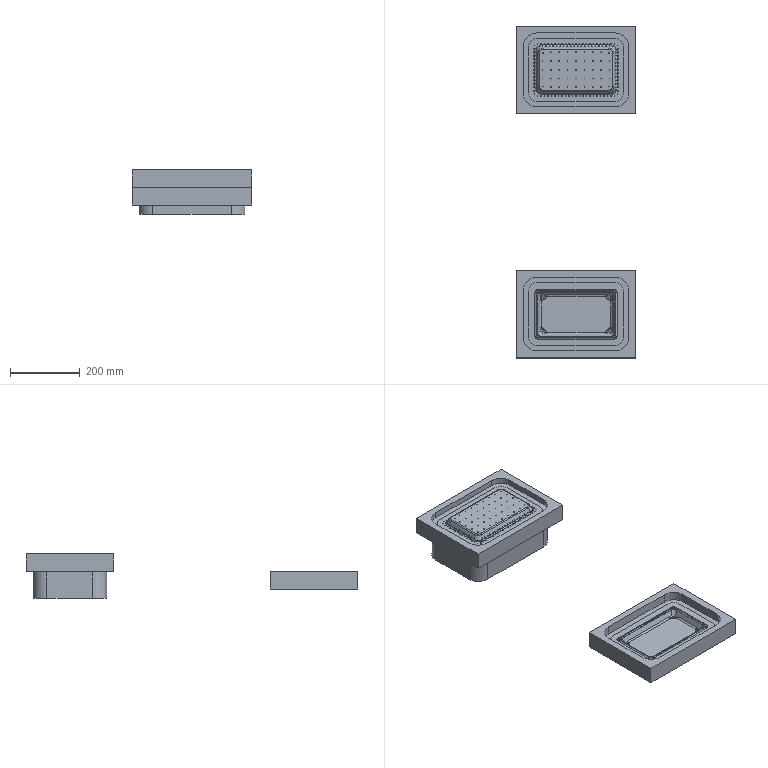NC program | NX | posted with a generic post | part box 343.99 x 952.259 x 127.368 mm
Lines 13466 to 14186 of 51088:
(CONTOUR_AREA_3 , TOOL : R2)
N26912 M6
N26914 G53
N26916 G17 G0 G90 X61.377 Y-421.815 S9000 M3 M8
N26918 G43 Z150. H0
N26920 Z-20.4
N26922 G94 G1 Z-25.125 F4000.
N26924 G2 X54.285 Y-414.412 R8.003
N26926 G1 X54.273 Y-414.066 Z-25.128
N26928 X54.264 Y-413.72
N26930 X54.26 Y-399.601
N26932 Y-287.414
N26934 X54.272 Y-287.07
N26936 X54.284 Y-286.727 Z-25.126
N26938 G2 X55.837 Y-282.505 R8.051
N26940 G1 X55.9 Y-282.423 Z-25.122
N26942 X56.055 Y-282.221 Z-25.126
N26944 G2 X61.723 Y-279.282 R8.023
N26946 G1 X62.069 Y-279.272 Z-25.128
N26948 X62.415 Y-279.262
N26950 X281.574 Y-279.265
N26952 X281.91 Y-279.272
N26954 X282.257 Y-279.282 Z-25.126
N26956 G2 X289.705 Y-286.717 R8.004
N26958 G1 X289.717 Y-287.063 Z-25.128
N26960 X289.73 Y-287.409
N26962 Y-413.374
N26964 X289.726 Y-413.72
N26966 X289.718 Y-414.059
N26968 X289.706 Y-414.402 Z-25.126
N26970 G2 X288.43 Y-418.219 R7.954
N26972 G1 X288.271 Y-418.455 Z-25.122
N26974 X288.196 Y-418.564 Z-25.126
N26976 G2 X282.267 Y-421.847 R8.033
N26978 G1 X281.23 Y-421.867 Z-25.128
N26980 X62.418
N26982 X62.08 Y-421.857
N26984 X61.733 Y-421.847 Z-25.126
N26986 X61.377 Y-421.815 Z-25.125
N26988 X61.394 Y-421.679 Z-25.115
N26990 X61.4 Y-421.633 Z-25.102
N26992 X61.413 Y-421.534 Z-25.077
N26994 X61.377 Y-421.529 Z-25.078
N26996 X61.204 Y-421.506 Z-25.074
N26998 X60.684 Y-421.42 Z-25.083
N27000 X60.331 Y-421.333 Z-25.091
N27002 X60.065 Y-421.26 Z-25.079
N27004 X59.992 Y-421.237 Z-25.082
N27006 X59.802 Y-421.177 Z-25.07
N27008 X59.646 Y-421.121 Z-25.082
N27010 X59.571 Y-421.095 Z-25.08
N27012 X59.493 Y-421.064 Z-25.084
N27014 X59.304 Y-420.987 Z-25.089
N27016 X59.059 Y-420.882 Z-25.072
N27018 X58.953 Y-420.831 Z-25.081
N27020 X58.759 Y-420.738
N27022 X58.577 Y-420.641 Z-25.088
N27024 X58.261 Y-420.456 Z-25.09
N27026 X58.008 Y-420.295 Z-25.088
N27028 X57.951 Y-420.259 Z-25.081
N27030 X57.915 Y-420.231 Z-25.085
N27032 X57.746 Y-420.118 Z-25.067
N27034 X57.568 Y-419.985 Z-25.088
N27036 X57.537 Y-419.961
N27038 X57.522 Y-419.949
N27040 X57.353 Y-419.818 Z-25.067
N27042 X57.222 Y-419.702 Z-25.085
N27044 X57.049 Y-419.548 Z-25.088
N27046 X56.948 Y-419.458 Z-25.076
N27048 X56.876 Y-419.386 Z-25.085
N27050 X56.831 Y-419.342 Z-25.081
N27052 X56.791 Y-419.302
N27054 X56.747 Y-419.257 Z-25.085
N27056 X56.639 Y-419.148 Z-25.069
N27058 X56.53 Y-419.024 Z-25.087
N27060 X56.431 Y-418.911 Z-25.085
N27062 X56.315 Y-418.779 Z-25.067
N27064 X56.183 Y-418.61 Z-25.088
N27066 X56.172 Y-418.596
N27068 X56.149 Y-418.565
N27070 X56.015 Y-418.387 Z-25.067
N27072 X55.9 Y-418.219 Z-25.085
N27074 X55.873 Y-418.183 Z-25.081
N27076 X55.837 Y-418.126 Z-25.088
N27078 X55.613 Y-417.771 Z-25.091
N27080 X55.453 Y-417.489 Z-25.089
N27082 X55.302 Y-417.181 Z-25.08
N27084 X55.25 Y-417.075 Z-25.072
N27086 X55.145 Y-416.83 Z-25.089
N27088 X55.068 Y-416.642 Z-25.084
N27090 X55.038 Y-416.566 Z-25.08
N27092 X55.011 Y-416.488 Z-25.082
N27094 X54.954 Y-416.333 Z-25.07
N27096 X54.895 Y-416.142 Z-25.082
N27098 X54.871 Y-416.07 Z-25.079
N27100 X54.799 Y-415.805 Z-25.091
N27102 X54.713 Y-415.45 Z-25.083
N27104 X54.671 Y-415.232 Z-25.077
N27106 X54.65 Y-415.104 Z-25.079
N27108 X54.623 Y-414.933 Z-25.074
N27110 X54.602 Y-414.758 Z-25.077
N27112 X54.586 Y-414.624 Z-25.076
N27114 X54.57 Y-414.412 Z-25.08
N27116 X54.563 Y-414.302 Z-25.079
N27118 X54.543 Y-413.63 Z-25.086
N27120 X54.546 Y-287.409 Z-25.085
N27122 X54.57 Y-286.717 Z-25.08
N27124 X54.586 Y-286.505 Z-25.076
N27126 X54.602 Y-286.371 Z-25.077
N27128 X54.624 Y-286.196 Z-25.074
N27130 X54.65 Y-286.025 Z-25.079
N27132 X54.671 Y-285.898 Z-25.077
N27134 X54.74 Y-285.562 Z-25.085
N27136 X54.799 Y-285.324 Z-25.091
N27138 X54.871 Y-285.06 Z-25.079
N27140 X54.895 Y-284.987 Z-25.082
N27142 X54.954 Y-284.797 Z-25.07
N27144 X55.011 Y-284.641 Z-25.082
N27146 X55.037 Y-284.566 Z-25.08
N27148 X55.068 Y-284.488 Z-25.084
N27150 X55.145 Y-284.299 Z-25.089
N27152 X55.25 Y-284.054 Z-25.072
N27154 X55.301 Y-283.949 Z-25.081
N27156 X55.394 Y-283.755
N27158 X55.491 Y-283.572 Z-25.088
N27160 X55.676 Y-283.257 Z-25.09
N27162 X55.837 Y-283.004 Z-25.088
N27164 X55.873 Y-282.947 Z-25.081
N27166 X55.901 Y-282.911 Z-25.085
N27168 X56.015 Y-282.742 Z-25.067
N27170 X56.172 Y-282.533 Z-25.088
N27172 X56.183 Y-282.518
N27174 X56.315 Y-282.35 Z-25.067
N27176 X56.431 Y-282.219 Z-25.085
N27178 X56.632 Y-281.994 Z-25.091
N27180 X56.831 Y-281.787 Z-25.081
N27182 X57.222 Y-281.429 Z-25.09
N27184 X57.437 Y-281.246 Z-25.091
N27186 X57.568 Y-281.146 Z-25.088
N27188 X57.746 Y-281.012 Z-25.067
N27190 X57.915 Y-280.897 Z-25.085
N27192 X57.951 Y-280.87 Z-25.081
N27194 X58.008 Y-280.834 Z-25.089
N27196 X58.18 Y-280.721 Z-25.077
N27198 X58.261 Y-280.672 Z-25.083
N27200 X58.374 Y-280.601 Z-25.07
N27202 X58.607 Y-280.472 Z-25.088
N27204 X58.738 Y-280.403 Z-25.084
N27206 X58.909 Y-280.319
N27208 X59.058 Y-280.247 Z-25.072
N27210 X59.304 Y-280.142 Z-25.089
N27212 X59.493 Y-280.066 Z-25.084
N27214 X59.568 Y-280.036 Z-25.08
N27216 X59.646 Y-280.008 Z-25.082
N27218 X59.802 Y-279.952 Z-25.07
N27220 X59.992 Y-279.892 Z-25.082
N27222 X60.065 Y-279.869 Z-25.079
N27224 X60.331 Y-279.796 Z-25.091
N27226 X60.684 Y-279.712 Z-25.083
N27228 X60.907 Y-279.672 Z-25.077
N27230 X61.031 Y-279.653 Z-25.079
N27232 X61.206 Y-279.625 Z-25.073
N27234 X61.377 Y-279.602 Z-25.077
N27236 X61.512 Y-279.585 Z-25.076
N27238 X61.723 Y-279.568 Z-25.08
N27240 X61.834 Y-279.561
N27242 X62.668 Y-279.544 Z-25.085
N27244 X281.574 Y-279.546
N27246 X282.267 Y-279.568 Z-25.08
N27248 X282.478 Y-279.585 Z-25.076
N27250 X282.613 Y-279.602 Z-25.077
N27252 X282.784 Y-279.625 Z-25.073
N27254 X283.334 Y-279.717 Z-25.082
N27256 X283.422 Y-279.738 Z-25.085
N27258 X283.659 Y-279.796 Z-25.091
N27260 X283.925 Y-279.869 Z-25.079
N27262 X283.998 Y-279.892 Z-25.082
N27264 X284.188 Y-279.952 Z-25.07
N27266 X284.344 Y-280.008 Z-25.082
N27268 X284.419 Y-280.035 Z-25.08
N27270 X284.497 Y-280.066 Z-25.084
N27272 X284.686 Y-280.142 Z-25.089
N27274 X284.931 Y-280.247 Z-25.072
N27276 X285.037 Y-280.298 Z-25.081
N27278 X285.231 Y-280.391
N27280 X285.413 Y-280.488 Z-25.088
N27282 X285.616 Y-280.601 Z-25.07
N27284 X285.729 Y-280.673 Z-25.083
N27286 X285.809 Y-280.721 Z-25.077
N27288 X285.981 Y-280.834 Z-25.088
N27290 X286.039 Y-280.871 Z-25.081
N27292 X286.075 Y-280.898 Z-25.085
N27294 X286.244 Y-281.012 Z-25.067
N27296 X286.467 Y-281.18 Z-25.09
N27298 X286.682 Y-281.354 Z-25.091
N27300 X286.768 Y-281.429 Z-25.09
N27302 X287.159 Y-281.787 Z-25.081
N27304 X287.199 Y-281.827
N27306 X287.243 Y-281.872 Z-25.085
N27308 X287.351 Y-281.981 Z-25.069
N27310 X287.46 Y-282.106 Z-25.087
N27312 X287.496 Y-282.146 Z-25.084
N27314 X287.532 Y-282.187
N27316 X287.632 Y-282.305 Z-25.091
N27318 X287.841 Y-282.565 Z-25.088
N27320 X287.975 Y-282.742 Z-25.067
N27322 X288.09 Y-282.911 Z-25.085
N27324 X288.117 Y-282.946 Z-25.081
N27326 X288.153 Y-283.004 Z-25.088
N27328 X288.266 Y-283.176 Z-25.077
N27330 X288.315 Y-283.257 Z-25.083
N27332 X288.386 Y-283.37 Z-25.07
N27334 X288.516 Y-283.603 Z-25.088
N27336 X288.57 Y-283.705 Z-25.086
N27338 X288.641 Y-283.847
N27340 X288.69 Y-283.949 Z-25.081
N27342 X288.74 Y-284.054 Z-25.072
N27344 X288.844 Y-284.297 Z-25.088
N27346 X288.922 Y-284.488 Z-25.084
N27348 X288.951 Y-284.563 Z-25.08
N27350 X288.979 Y-284.641 Z-25.082
N27352 X289.036 Y-284.797 Z-25.07
N27354 X289.095 Y-284.987 Z-25.082
N27356 X289.119 Y-285.06 Z-25.079
N27358 X289.191 Y-285.324 Z-25.091
N27360 X289.277 Y-285.679 Z-25.083
N27362 X289.319 Y-285.898 Z-25.077
N27364 X289.34 Y-286.025 Z-25.079
N27366 X289.367 Y-286.196 Z-25.074
N27368 X289.389 Y-286.371 Z-25.078
N27370 X289.398 Y-286.441 Z-25.076
N27372 X289.427 Y-286.827 Z-25.079
N27374 X289.447 Y-287.5 Z-25.086
N27376 X289.444 Y-413.72 Z-25.085
N27378 X289.421 Y-414.412 Z-25.08
N27380 X289.389 Y-414.758 Z-25.078
N27382 X289.367 Y-414.933 Z-25.074
N27384 X289.34 Y-415.104 Z-25.079
N27386 X289.319 Y-415.232 Z-25.077
N27388 X289.25 Y-415.568 Z-25.085
N27390 X289.191 Y-415.805 Z-25.091
N27392 X289.119 Y-416.07 Z-25.079
N27394 X289.095 Y-416.142 Z-25.082
N27396 X289.036 Y-416.333 Z-25.07
N27398 X288.979 Y-416.488 Z-25.082
N27400 X288.953 Y-416.563 Z-25.08
N27402 X288.922 Y-416.642 Z-25.084
N27404 X288.845 Y-416.83 Z-25.089
N27406 X288.74 Y-417.075 Z-25.072
N27408 X288.69 Y-417.181 Z-25.081
N27410 X288.668 Y-417.225 Z-25.084
N27412 X288.536 Y-417.489 Z-25.089
N27414 X288.516 Y-417.526 Z-25.088
N27416 X288.515 Y-417.527
N27418 X288.386 Y-417.76 Z-25.07
N27420 X288.313 Y-417.873 Z-25.082
N27422 X288.153 Y-418.125 Z-25.088
N27424 X288.117 Y-418.183 Z-25.081
N27426 X288.09 Y-418.219 Z-25.085
N27428 X287.975 Y-418.387 Z-25.067
N27430 X287.841 Y-418.565 Z-25.088
N27432 X287.818 Y-418.595 Z-25.087
N27434 X287.806 Y-418.61 Z-25.088
N27436 X287.675 Y-418.779 Z-25.067
N27438 X287.559 Y-418.911 Z-25.085
N27440 X287.358 Y-419.135 Z-25.091
N27442 X287.159 Y-419.342 Z-25.081
N27444 X286.84 Y-419.639 Z-25.084
N27446 X286.768 Y-419.7 Z-25.09
N27448 X286.554 Y-419.883 Z-25.092
N27450 X286.371 Y-420.023 Z-25.088
N27452 X286.312 Y-420.067 Z-25.081
N27454 X286.075 Y-420.232 Z-25.085
N27456 X286.039 Y-420.259 Z-25.081
N27458 X285.982 Y-420.295 Z-25.088
N27460 X285.81 Y-420.408 Z-25.077
N27462 X285.729 Y-420.457 Z-25.083
N27464 X285.616 Y-420.528 Z-25.071
N27466 X285.383 Y-420.658 Z-25.088
N27468 X285.231 Y-420.738 Z-25.081
N27470 X285.037 Y-420.831
N27472 X284.931 Y-420.882 Z-25.072
N27474 X284.686 Y-420.987 Z-25.089
N27476 X284.497 Y-421.064 Z-25.084
N27478 X284.422 Y-421.093 Z-25.08
N27480 X284.344 Y-421.121 Z-25.082
N27482 X284.188 Y-421.178 Z-25.07
N27484 X283.998 Y-421.237 Z-25.082
N27486 X283.925 Y-421.26 Z-25.079
N27488 X283.659 Y-421.333 Z-25.091
N27490 X283.306 Y-421.417 Z-25.083
N27492 X283.083 Y-421.457 Z-25.077
N27494 X282.959 Y-421.476 Z-25.079
N27496 X282.784 Y-421.504 Z-25.073
N27498 X282.613 Y-421.527 Z-25.077
N27500 X282.478 Y-421.544 Z-25.076
N27502 X282.267 Y-421.561 Z-25.08
N27504 X282.156 Y-421.568
N27506 X281.322 Y-421.585 Z-25.085
N27508 X62.415 Y-421.584
N27510 X61.723 Y-421.563 Z-25.08
N27512 X61.413 Y-421.534 Z-25.077
N27514 X61.437 Y-421.333 Z-25.026
N27516 X61.446 Y-421.265 Z-24.985
N27518 X61.377 Y-421.257 Z-24.984
N27520 X61.139 Y-421.225 Z-24.98
N27522 X61.031 Y-421.206 Z-24.984
N27524 X60.84 Y-421.177 Z-24.979
N27526 X60.684 Y-421.145 Z-24.984
N27528 X60.554 Y-421.117 Z-24.979
N27530 X60.338 Y-421.058 Z-24.99
N27532 X60.282 Y-421.043 Z-24.988
N27534 X60.101 Y-420.987 Z-24.996
N27536 X60.016 Y-420.963 Z-24.988
N27538 X59.958 Y-420.941 Z-24.992
N27540 X59.68 Y-420.848 Z-24.985
N27542 X59.646 Y-420.835 Z-24.986
N27544 X59.503 Y-420.785 Z-24.975
N27546 X59.3 Y-420.691 Z-24.992
N27548 X58.825 Y-420.468 Z-24.997
N27550 X58.515 Y-420.295 Z-24.998
N27552 X58.294 Y-420.163 Z-24.986
N27554 X58.261 Y-420.141 Z-24.987
N27556 X58.162 Y-420.083 Z-24.975
N27558 X58.14 Y-420.07 Z-24.972
N27560 X57.981 Y-419.949 Z-24.992
N27562 X57.915 Y-419.901 Z-24.994
N27564 X57.74 Y-419.775 Z-24.998
N27566 X57.568 Y-419.64 Z-24.994
N27568 X57.548 Y-419.624 Z-24.992
N27570 X57.524 Y-419.603 Z-24.995
N27572 X57.222 Y-419.34 Z-24.994
N27574 X57.134 Y-419.257 Z-24.996
N27576 X56.968 Y-419.094 Z-24.997
N27578 X56.876 Y-418.999 Z-24.994
N27580 X56.832 Y-418.955 Z-24.987
N27582 X56.794 Y-418.911 Z-24.993
N27584 X56.493 Y-418.565 Z-24.994
N27586 X56.304 Y-418.324 Z-24.985
N27588 X56.23 Y-418.219 Z-24.994
N27590 X56.183 Y-418.154 Z-24.993
N27592 X56.063 Y-417.994 Z-24.972
N27594 X55.991 Y-417.873 Z-24.986
N27596 X55.952 Y-417.815 Z-24.982
N27598 X55.837 Y-417.619 Z-24.997
N27600 X55.633 Y-417.244 Z-24.991
N27602 X55.603 Y-417.181 Z-24.995
N27604 X55.491 Y-416.942
N27606 X55.456 Y-416.869 Z-24.989
N27608 X55.441 Y-416.834 Z-24.992
N27610 X55.383 Y-416.716 Z-24.98
N27612 X55.334 Y-416.583 Z-24.989
N27614 X55.297 Y-416.488 Z-24.986
N27616 X55.253 Y-416.38 Z-24.977
N27618 X55.165 Y-416.102 Z-24.991
N27620 X55.145 Y-416.035 Z-24.995
N27622 X55.089 Y-415.853 Z-24.987
N27624 X55.074 Y-415.796 Z-24.989
N27626 X55.015 Y-415.58 Z-24.978
N27628 X54.987 Y-415.45 Z-24.983
N27630 X54.968 Y-415.366 Z-24.98
N27632 X54.934 Y-415.172 Z-24.986
N27634 X54.922 Y-415.104 Z-24.985
N27636 X54.904 Y-414.999 Z-24.981
N27638 X54.872 Y-414.758 Z-24.985
N27640 X54.864 Y-414.693 Z-24.984
N27642 X54.839 Y-414.412 Z-24.989
N27644 X54.836 Y-414.375
N27646 X54.824 Y-414.066 Z-24.991
N27648 X54.812 Y-413.72 Z-24.994
N27650 X54.815 Y-287.409 Z-24.992
N27652 X54.84 Y-286.696 Z-24.989
N27654 X54.867 Y-286.405 Z-24.984
N27656 X54.872 Y-286.371 Z-24.985
N27658 X54.904 Y-286.13 Z-24.981
N27660 X54.923 Y-286.025 Z-24.984
N27662 X54.954 Y-285.834 Z-24.979
N27664 X54.988 Y-285.679 Z-24.983
N27666 X55.015 Y-285.549 Z-24.978
N27668 X55.073 Y-285.333 Z-24.99
N27670 X55.089 Y-285.277 Z-24.987
N27672 X55.145 Y-285.094 Z-24.995
N27674 X55.19 Y-284.953 Z-24.992
N27676 X55.284 Y-284.676 Z-24.985
N27678 X55.297 Y-284.641 Z-24.986
N27680 X55.346 Y-284.498 Z-24.974
N27682 X55.441 Y-284.295 Z-24.992
N27684 X55.631 Y-283.882
N27686 X55.715 Y-283.714 Z-24.98
N27688 X55.783 Y-283.603 Z-24.994
N27690 X55.812 Y-283.552
N27692 X55.837 Y-283.51 Z-24.997
N27694 X55.969 Y-283.29 Z-24.985
N27696 X55.991 Y-283.257 Z-24.986
N27698 X56.049 Y-283.158 Z-24.975
N27700 X56.063 Y-283.136 Z-24.972
N27702 X56.183 Y-282.978 Z-24.992
N27704 X56.217 Y-282.927 Z-24.989
N27706 X56.231 Y-282.911 Z-24.991
N27708 X56.351 Y-282.732 Z-24.97
N27710 X56.493 Y-282.565 Z-24.994
N27712 X56.792 Y-282.219
N27714 X56.876 Y-282.129
N27716 X57.134 Y-281.872
N27718 X57.222 Y-281.79 Z-24.996
N27720 X57.268 Y-281.746 Z-24.992
N27722 X57.568 Y-281.487 Z-24.995
N27724 X57.738 Y-281.357 Z-24.998
N27726 X57.915 Y-281.227 Z-24.994
N27728 X57.98 Y-281.18 Z-24.993
N27730 X58.14 Y-281.06 Z-24.972
N27732 X58.261 Y-280.99 Z-24.986
N27734 X58.319 Y-280.95 Z-24.981
N27736 X58.519 Y-280.834 Z-24.997
N27738 X58.573 Y-280.8 Z-24.991
N27740 X58.726 Y-280.715 Z-24.999
N27742 X58.953 Y-280.595 Z-24.988
N27744 X59.022 Y-280.557 Z-24.981
N27746 X59.192 Y-280.488 Z-24.996
N27748 X59.501 Y-280.345 Z-24.975
N27750 X59.646 Y-280.295 Z-24.986
N27752 X59.754 Y-280.251 Z-24.978
N27754 X59.992 Y-280.176 Z-24.99
N27756 X60.016 Y-280.166 Z-24.988
N27758 X60.101 Y-280.142 Z-24.996
N27760 X60.282 Y-280.086 Z-24.988
N27762 X60.338 Y-280.072 Z-24.99
N27764 X60.555 Y-280.013 Z-24.978
N27766 X60.684 Y-279.986 Z-24.983
N27768 X60.77 Y-279.967 Z-24.979
N27770 X60.961 Y-279.936 Z-24.984
N27772 X61.031 Y-279.925 Z-24.983
N27774 X61.14 Y-279.906 Z-24.979
N27776 X61.377 Y-279.872 Z-24.984
N27778 X61.412 Y-279.866 Z-24.983
N27780 X61.761 Y-279.834 Z-24.99
N27782 X62.069 Y-279.824
N27784 X62.415 Y-279.816 Z-24.991
N27786 X281.574 Y-279.814 Z-24.993
N27788 X282.288 Y-279.838 Z-24.989
N27790 X282.578 Y-279.866 Z-24.983
N27792 X282.613 Y-279.872 Z-24.984
N27794 X282.85 Y-279.906 Z-24.979
N27796 X282.959 Y-279.925 Z-24.983
N27798 X283.148 Y-279.954 Z-24.978
N27800 X283.306 Y-279.987 Z-24.983
N27802 X283.435 Y-280.013 Z-24.978
N27804 X283.652 Y-280.071 Z-24.99
N27806 X283.707 Y-280.086 Z-24.988
N27808 X283.889 Y-280.142 Z-24.996
N27810 X283.974 Y-280.166 Z-24.988
N27812 X284.032 Y-280.188 Z-24.992
N27814 X284.309 Y-280.281 Z-24.985
N27816 X284.344 Y-280.294 Z-24.986
N27818 X284.487 Y-280.344 Z-24.975
N27820 X284.69 Y-280.438 Z-24.992
N27822 X285.103 Y-280.628
N27824 X285.271 Y-280.712 Z-24.979
N27826 X285.383 Y-280.782 Z-24.994
N27828 X285.417 Y-280.801 Z-24.991
N27830 X285.471 Y-280.834 Z-24.997
N27832 X285.696 Y-280.968 Z-24.985
N27834 X285.729 Y-280.989 Z-24.986
N27836 X285.828 Y-281.046 Z-24.975
N27838 X285.85 Y-281.06 Z-24.972
N27840 X286.008 Y-281.18 Z-24.992
N27842 X286.059 Y-281.214 Z-24.989
N27844 X286.075 Y-281.228 Z-24.991
N27846 X286.255 Y-281.347 Z-24.97
N27848 X286.422 Y-281.489 Z-24.994
N27850 X286.468 Y-281.526 Z-24.995
N27852 X286.534 Y-281.583 Z-24.998
N27854 X286.768 Y-281.791 Z-24.996
N27856 X286.856 Y-281.872 Z-24.994
N27858 X287.114 Y-282.13
N27860 X287.158 Y-282.174 Z-24.987
N27862 X287.196 Y-282.219 Z-24.993
N27864 X287.46 Y-282.519 Z-24.995
N27866 X287.498 Y-282.565 Z-24.994
N27868 X287.686 Y-282.805 Z-24.985
N27870 X287.76 Y-282.911 Z-24.994
N27872 X287.806 Y-282.976 Z-24.993
N27874 X287.927 Y-283.136 Z-24.972
N27876 X287.997 Y-283.257 Z-24.986
N27878 X288.037 Y-283.314 Z-24.981
N27880 X288.153 Y-283.514 Z-24.997
N27882 X288.187 Y-283.569 Z-24.991
N27884 X288.273 Y-283.723 Z-24.999
N27886 X288.392 Y-283.949 Z-24.988
N27888 X288.43 Y-284.018 Z-24.98
N27890 X288.499 Y-284.187 Z-24.995
N27892 X288.534 Y-284.26 Z-24.989
N27894 X288.548 Y-284.295 Z-24.991
N27896 X288.682 Y-284.62 Z-24.996
N27898 X288.69 Y-284.641 Z-24.997
N27900 X288.825 Y-285.027 Z-24.992
N27902 X288.845 Y-285.094 Z-24.995
N27904 X288.901 Y-285.277 Z-24.987
N27906 X288.916 Y-285.333 Z-24.989
N27908 X288.975 Y-285.549 Z-24.978
N27910 X289.003 Y-285.679 Z-24.983
N27912 X289.022 Y-285.763 Z-24.98
N27914 X289.056 Y-285.957 Z-24.986
N27916 X289.068 Y-286.025 Z-24.985
N27918 X289.086 Y-286.13 Z-24.981
N27920 X289.14 Y-286.57 Z-24.984
N27922 X289.151 Y-286.717 Z-24.989
N27924 X289.154 Y-286.755
N27926 X289.166 Y-287.063 Z-24.991
N27928 X289.178 Y-287.423 Z-24.994
N27930 Y-413.72
N27932 X289.151 Y-414.412 Z-24.989
N27934 X289.14 Y-414.559 Z-24.984
N27936 X289.134 Y-414.614 Z-24.986
N27938 X289.117 Y-414.758 Z-24.984
N27940 X289.086 Y-414.999 Z-24.981
N27942 X289.067 Y-415.104 Z-24.984
N27944 X289.036 Y-415.295 Z-24.979
N27946 X289.002 Y-415.45 Z-24.983
N27948 X288.975 Y-415.58 Z-24.978
N27950 X288.917 Y-415.796 Z-24.99
N27952 X288.901 Y-415.852 Z-24.987
N27954 X288.845 Y-416.035 Z-24.995
N27956 X288.825 Y-416.102 Z-24.991
N27958 X288.737 Y-416.38 Z-24.977
N27960 X288.692 Y-416.488 Z-24.986
N27962 X288.643 Y-416.631 Z-24.974
N27964 X288.549 Y-416.834 Z-24.992
N27966 X288.534 Y-416.869 Z-24.989
N27968 X288.499 Y-416.942 Z-24.995
N27970 X288.429 Y-417.111 Z-24.98
N27972 X288.391 Y-417.181 Z-24.987
N27974 X288.366 Y-417.234 Z-24.985
N27976 X288.326 Y-417.31 Z-24.989
N27978 X288.275 Y-417.415 Z-24.979
N27980 X288.205 Y-417.527 Z-24.994
N27982 X288.187 Y-417.56 Z-24.991
N27984 X288.153 Y-417.615 Z-24.996
N27986 X288.02 Y-417.839 Z-24.985
N27988 X287.998 Y-417.873 Z-24.986
N27990 X287.941 Y-417.971 Z-24.975
N27992 X287.928 Y-417.994 Z-24.972
N27994 X287.806 Y-418.153 Z-24.993
N27996 X287.76 Y-418.219 Z-24.991
N27998 X287.639 Y-418.398 Z-24.97
N28000 X287.497 Y-418.565 Z-24.994
N28002 X287.198 Y-418.911
N28004 X287.114 Y-419.001
N28006 X286.856 Y-419.257
N28008 X286.469 Y-419.603 Z-24.996
N28010 X286.422 Y-419.642 Z-24.995
N28012 X286.245 Y-419.78 Z-24.999
N28014 X286.075 Y-419.903 Z-24.994
N28016 X286.01 Y-419.949 Z-24.993
N28018 X285.85 Y-420.069 Z-24.972
N28020 X285.729 Y-420.14 Z-24.986
N28022 X285.671 Y-420.179 Z-24.981
N28024 X285.471 Y-420.295 Z-24.997
N28026 X285.417 Y-420.329 Z-24.991
N28028 X285.383 Y-420.347 Z-24.994
N28030 X285.102 Y-420.501 Z-24.992
N28032 X285.037 Y-420.531 Z-24.996
N28034 X284.798 Y-420.641
N28036 X284.489 Y-420.785 Z-24.975
N28038 X284.344 Y-420.835 Z-24.986
N28040 X284.309 Y-420.848 Z-24.985
N28042 X284.032 Y-420.941 Z-24.992
N28044 X283.974 Y-420.963 Z-24.988
N28046 X283.889 Y-420.987 Z-24.996
N28048 X283.708 Y-421.043 Z-24.988
N28050 X283.652 Y-421.057 Z-24.99
N28052 X283.435 Y-421.116 Z-24.978
N28054 X283.306 Y-421.143 Z-24.983
N28056 X283.148 Y-421.175 Z-24.978
N28058 X282.959 Y-421.204 Z-24.983
N28060 X282.85 Y-421.224 Z-24.979
N28062 X282.613 Y-421.257 Z-24.984
N28064 X282.578 Y-421.263 Z-24.983
N28066 X282.229 Y-421.295 Z-24.99
N28068 X281.921 Y-421.306
N28070 X281.574 Y-421.313 Z-24.991
N28072 X62.433 Y-421.316 Z-24.993
N28074 X61.723 Y-421.293 Z-24.989
N28076 X61.446 Y-421.265 Z-24.985
N28078 X61.459 Y-421.152 Z-24.917
N28080 X61.475 Y-421.023 Z-24.837
N28082 X61.031 Y-420.956 Z-24.84
N28084 X60.815 Y-420.922 Z-24.836
N28086 X60.684 Y-420.898 Z-24.83
N28088 X60.472 Y-420.853 Z-24.822
N28090 X60.338 Y-420.812 Z-24.829
N28092 X60.237 Y-420.788 Z-24.824
N28094 X60.2 Y-420.779 Z-24.822
N28096 X59.997 Y-420.703 Z-24.836
N28098 X59.838 Y-420.641 Z-24.844
N28100 X59.646 Y-420.578 Z-24.834
N28102 X59.526 Y-420.522 Z-24.841
N28104 X59.299 Y-420.43 Z-24.834
N28106 X59.158 Y-420.366 Z-24.836
N28108 X59.022 Y-420.295 Z-24.847
N28110 X58.953 Y-420.263 Z-24.842
N28112 X58.823 Y-420.209 Z-24.827
N28114 X58.693 Y-420.122 Z-24.84
N28116 X58.607 Y-420.072 Z-24.837
N28118 X58.419 Y-419.949 Z-24.843
N28120 X58.356 Y-419.914 Z-24.837
N28122 X58.347 Y-419.906 Z-24.839
N28124 X58.334 Y-419.896 Z-24.84
N28126 X58.261 Y-419.854 Z-24.831
N28128 X57.997 Y-419.669 Z-24.837
N28130 X57.916 Y-419.603 Z-24.847
N28132 X57.911 Y-419.599 Z-24.848
N28134 X57.568 Y-419.325 Z-24.839
N28136 X57.494 Y-419.257 Z-24.843
N28138 X57.314 Y-419.095 Z-24.844
N28140 X57.222 Y-419.011 Z-24.838
N28142 X57.123 Y-418.911 Z-24.837
N28144 X56.876 Y-418.64 Z-24.839
N28146 X56.81 Y-418.565 Z-24.838
N28148 X56.53 Y-418.213 Z-24.845
N28150 X56.478 Y-418.148 Z-24.841
N28152 X56.455 Y-418.121 Z-24.837
N28154 X56.337 Y-417.949 Z-24.839
N28156 X56.278 Y-417.873 Z-24.831
N28158 X56.168 Y-417.692 Z-24.843
N28160 X56.062 Y-417.527 Z-24.835
N28162 X55.918 Y-417.262 Z-24.845
N28164 X55.871 Y-417.181 Z-24.84
N28166 X55.854 Y-417.147
N28168 X55.837 Y-417.107 Z-24.844
N28170 X55.767 Y-416.975 Z-24.835
N28172 X55.701 Y-416.834 Z-24.834
N28174 X55.665 Y-416.748 Z-24.836
N28176 X55.607 Y-416.605 Z-24.842
N28178 X55.553 Y-416.488 Z-24.834
N28180 X55.528 Y-416.415 Z-24.836
N28182 X55.491 Y-416.301 Z-24.842
N28184 X55.446 Y-416.187 Z-24.833
N28186 X55.325 Y-415.783 Z-24.843
N28188 X55.234 Y-415.45 Z-24.83
N28190 X55.165 Y-415.064 Z-24.842
N28192 X55.145 Y-414.921 Z-24.844
N28194 X55.121 Y-414.781 Z-24.838
N28196 X55.119 Y-414.758
N28198 X55.08 Y-414.412 Z-24.833
N28200 X55.05 Y-413.722 Z-24.837
N28202 X55.051 Y-287.409 Z-24.836
N28204 X55.078 Y-286.725 Z-24.834
N28206 X55.092 Y-286.574 Z-24.833
N28208 X55.098 Y-286.521 Z-24.832
N28210 X55.145 Y-286.209 Z-24.843
N28212 X55.173 Y-286.025 Z-24.842
N28214 Y-286.011 Z-24.839
N28216 X55.221 Y-285.717 Z-24.826
N28218 X55.344 Y-285.281 Z-24.845
N28220 X55.431 Y-284.987 Z-24.836
N28222 X55.491 Y-284.832 Z-24.844
N28224 X55.554 Y-284.641 Z-24.833
N28226 X55.61 Y-284.522 Z-24.841
N28228 X55.702 Y-284.295 Z-24.833
N28230 X55.766 Y-284.153 Z-24.835
N28232 X55.837 Y-284.018 Z-24.846
N28234 X55.87 Y-283.949 Z-24.841
N28236 X55.925 Y-283.819 Z-24.826
N28238 X56.011 Y-283.689 Z-24.84
N28240 X56.06 Y-283.603 Z-24.837
N28242 X56.183 Y-283.415 Z-24.843
N28244 X56.236 Y-283.33 Z-24.839
N28246 X56.278 Y-283.257 Z-24.831
N28248 X56.337 Y-283.18 Z-24.838
N28250 X56.432 Y-283.035 Z-24.83
N28252 X56.547 Y-282.893 Z-24.846
N28254 X56.809 Y-282.565 Z-24.838
N28256 X56.876 Y-282.488 Z-24.84
N28258 X57.124 Y-282.219 Z-24.836
N28260 X57.222 Y-282.119 Z-24.837
N28262 X57.314 Y-282.035 Z-24.843
N28264 X57.493 Y-281.872 Z-24.844
N28266 X57.568 Y-281.804 Z-24.839
N28268 X57.91 Y-281.531 Z-24.848
N28270 X57.984 Y-281.474 Z-24.843
N28272 X58.012 Y-281.451 Z-24.838
N28274 X58.184 Y-281.334 Z-24.839
N28276 X58.261 Y-281.275 Z-24.831
N28278 X58.44 Y-281.168 Z-24.842
N28280 X58.607 Y-281.06 Z-24.835
N28282 X58.877 Y-280.91 Z-24.848
N28284 X58.953 Y-280.866 Z-24.842
N28286 X58.986 Y-280.85
N28288 X59.025 Y-280.834 Z-24.845
N28290 X59.203 Y-280.738 Z-24.826
N28292 X59.299 Y-280.7 Z-24.833
N28294 X59.527 Y-280.602 Z-24.834
N28296 X59.62 Y-280.568 Z-24.841
N28298 X59.646 Y-280.559 Z-24.842
N28300 X59.835 Y-280.488
N28302 X59.947 Y-280.443 Z-24.833
N28304 X59.992 Y-280.429 Z-24.835
N28306 X60.199 Y-280.349 Z-24.822
N28308 X60.338 Y-280.317 Z-24.829
N28310 X60.472 Y-280.276 Z-24.821
N28312 X60.908 Y-280.192 Z-24.836
N28314 X61.031 Y-280.175 Z-24.839
N28316 X61.245 Y-280.142 Z-24.841
N28318 X61.575 Y-280.092 Z-24.833
N28320 X61.719 Y-280.078 Z-24.835
N28322 X62.506 Y-280.052 Z-24.836
N28324 X281.702 Y-280.055 Z-24.834
N28326 X282.259 Y-280.077 Z-24.835
N28328 X282.411 Y-280.092 Z-24.833
N28330 X282.463 Y-280.097 Z-24.832
N28332 X282.745 Y-280.142 Z-24.841
N28334 X283.306 Y-280.233 Z-24.829
N28336 X283.517 Y-280.276 Z-24.821
N28338 X283.652 Y-280.317 Z-24.829
N28340 X283.753 Y-280.341 Z-24.824
N28342 X283.79 Y-280.35 Z-24.822
N28344 X283.993 Y-280.426 Z-24.836
N28346 X284.152 Y-280.488 Z-24.844